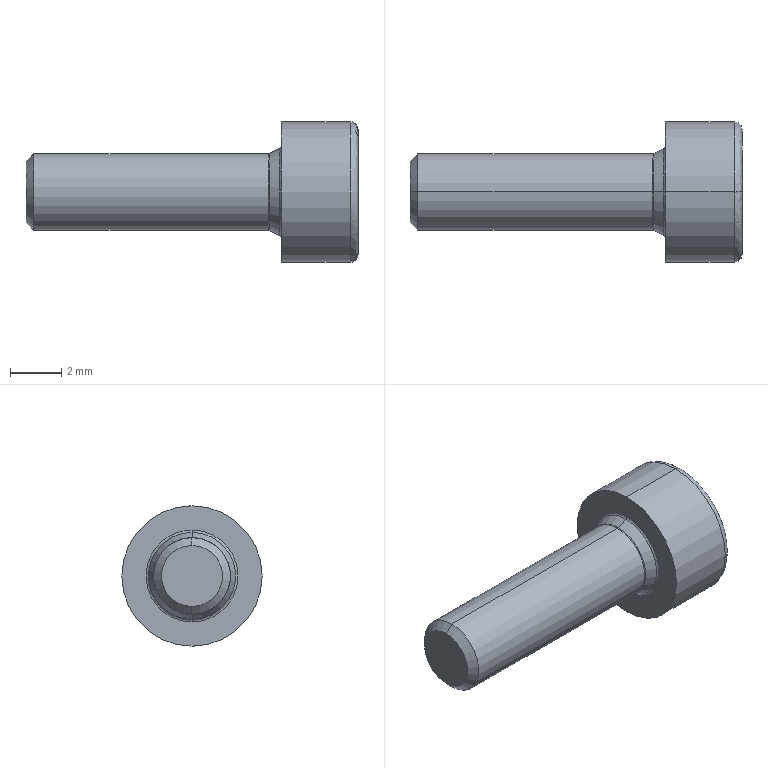Part | STEP file | PN_0001_Z_PSCLSJ10-14_2_Default | 1 solid | 31 faces | box 13 x 5.5 x 5.5 mm | volume 130.611 mm3 | plane 15 | spline 6 | cone 6 | cylinder 4 | commonest cylinder face diameters 3 x2 5.5 x2